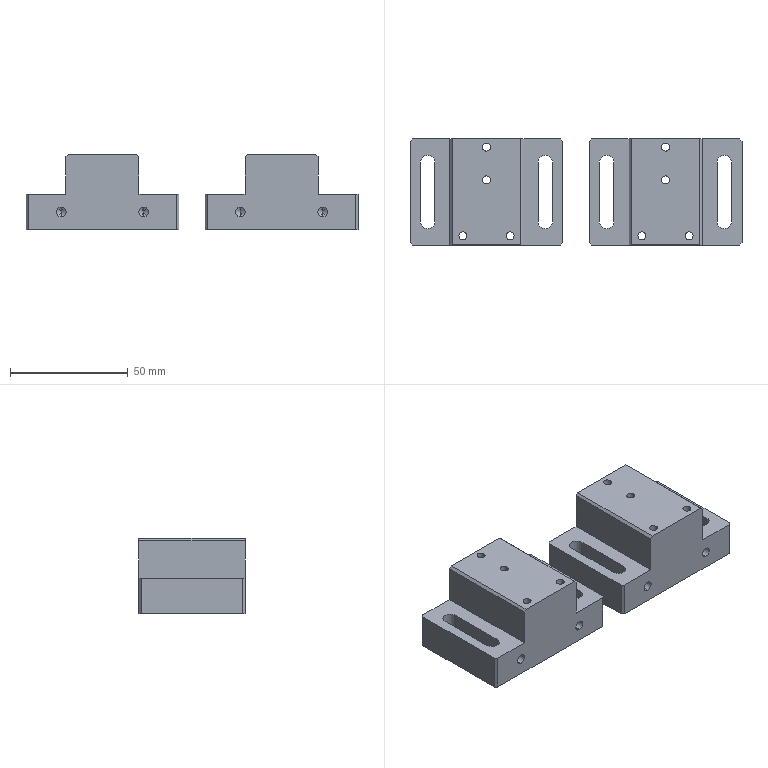NC program | NX | posted with a generic post | part box 140.92 x 45 x 32 mm
Lines 5945 to 6583 of 6583:
(FLOOR_WALL_1_COPY , TOOL : D10JING)
N11876 T14 M6
N11878 G54
N11880 G17 G0 G90 X-1.504 Y-6.448 S9500 M3
N11882 G43 Z30. H14
N11884 Z-15.5
N11886 G94 G1 Z-17. F1000.
N11888 X-0.497 Y-5.866
N11890 G3 X0.003 Y-5. R1.
N11892 G1 Y50. F1500.
N11894 X3.822
N11896 Y-5.
N11898 X7.641
N11900 Y50.
N11902 X11.46
N11904 Y-5.
N11906 G2 X10.96 Y-5.866 R1.
N11908 G1 X9.862 Y-6.5
N11910 Z-15.5
N11912 G0 X10.362
N11914 G1 Z-17. F1000.
N11916 X11.46 Y-5.866
N11918 G3 X11.96 Y-5. R1.
N11920 G1 Y50. F1500.
N11922 G3 X11.46 Y50.866 R1.
N11924 G1 X10.362 Y51.5
N11926 Z-15.5
N11928 G0 Z30.
N11930 X66.424 Y51.448
N11932 Z-15.5
N11934 G1 Z-17. F1000.
N11936 X65.417 Y50.866
N11938 G3 X64.917 Y50. R1.
N11940 G1 Y-5. F1500.
N11942 X61.098
N11944 Y50.
N11946 X57.279
N11948 Y-5.
N11950 X53.46
N11952 Y50.
N11954 G2 X53.96 Y50.866 R1.
N11956 G1 X55.058 Y51.5
N11958 Z-15.5
N11960 G0 X54.558
N11962 G1 Z-17. F1000.
N11964 X53.46 Y50.866
N11966 G3 X52.96 Y50. R1.
N11968 G1 Y-5. F1500.
N11970 G3 X53.46 Y-5.866 R1.
N11972 G1 X54.558 Y-6.5
N11974 Z-15.5
N11976 G0 Z30.
N11978 X74.496 Y-6.448
N11980 Z-15.5
N11982 G1 Z-17. F1000.
N11984 X75.503 Y-5.866
N11986 G3 X76.003 Y-5. R1.
N11988 G1 Y50. F1500.
N11990 X79.822
N11992 Y-5.
N11994 X83.641
N11996 Y50.
N11998 X87.46
N12000 Y-5.
N12002 G2 X86.96 Y-5.866 R1.
N12004 G1 X85.862 Y-6.5
N12006 Z-15.5
N12008 G0 X86.362
N12010 G1 Z-17. F1000.
N12012 X87.46 Y-5.866
N12014 G3 X87.96 Y-5. R1.
N12016 G1 Y50. F1500.
N12018 G3 X87.46 Y50.866 R1.
N12020 G1 X86.362 Y51.5
N12022 Z-15.5
N12024 G0 Z30.
N12026 X142.424 Y51.448
N12028 Z-15.5
N12030 G1 Z-17. F1000.
N12032 X141.417 Y50.866
N12034 G3 X140.917 Y50. R1.
N12036 G1 Y-5. F1500.
N12038 X137.098
N12040 Y50.
N12042 X133.279
N12044 Y-5.
N12046 X129.46
N12048 Y50.
N12050 G2 X129.96 Y50.866 R1.
N12052 G1 X131.058 Y51.5
N12054 Z-15.5
N12056 G0 X130.558
N12058 G1 Z-17. F1000.
N12060 X129.46 Y50.866
N12062 G3 X128.96 Y50. R1.
N12064 G1 Y-5. F1500.
N12066 G3 X129.46 Y-5.866 R1.
N12068 G1 X130.558 Y-6.5
N12070 Z-15.5
N12072 G0 Z30.
(ZLEVEL_PROFILE_1 , TOOL : D10JING)
N12074 X141.582 Y-6.809
N12076 Z-14.5
N12078 G1 Z-16. F1000.
N12080 X140.826 Y-5.5
N12082 G3 X139.96 Y-5. R1.
N12084 G1 X76.96 F1500.
N12086 G2 X73.424 Y-3.536 R5.
N12088 G1 X72.464 Y-2.576
N12090 G2 X71. Y0.96 R5.
N12092 G1 Y44.04
N12094 G2 X72.464 Y47.576 R5.
N12096 G1 X73.424 Y48.536
N12098 G2 X76.96 Y50. R5.
N12100 G1 X139.96
N12102 G2 X143.496 Y48.536 R5.
N12104 G1 X144.456 Y47.576
N12106 G2 X145.92 Y44.04 R5.
N12108 G1 Y0.96
N12110 G2 X144.456 Y-2.576 R5.
N12112 G1 X143.496 Y-3.536
N12114 G2 X139.96 Y-5. R5.
N12116 G3 X139.094 Y-5.5 R1.
N12118 G1 X138.228 Y-7.
N12120 Z-14.5
N12122 G0 Z30.
N12124 X65.582 Y-6.809
N12126 Z-14.5
N12128 G1 Z-16. F1000.
N12130 X64.826 Y-5.5
N12132 G3 X63.96 Y-5. R1.
N12134 G1 X0.96 F1500.
N12136 G2 X-2.576 Y-3.536 R5.
N12138 G1 X-3.536 Y-2.576
N12140 G2 X-5. Y0.96 R5.
N12142 G1 Y44.04
N12144 G2 X-3.536 Y47.576 R5.
N12146 G1 X-2.576 Y48.536
N12148 G2 X0.96 Y50. R5.
N12150 G1 X63.96
N12152 G2 X67.496 Y48.536 R5.
N12154 G1 X68.456 Y47.576
N12156 G2 X69.92 Y44.04 R5.
N12158 G1 Y0.96
N12160 G2 X68.456 Y-2.576 R5.
N12162 G1 X67.496 Y-3.536
N12164 G2 X63.96 Y-5. R5.
N12166 G1 X0.96 Z-20.048
N12168 X0.68 Y-4.992 Z-20.066
N12170 X0.4 Y-4.969 Z-20.084
N12172 X0.122 Y-4.929 Z-20.102
N12174 X-0.153 Y-4.875 Z-20.12
N12176 X-0.424 Y-4.805 Z-20.138
N12178 X-0.691 Y-4.719 Z-20.156
N12180 X-0.953 Y-4.619 Z-20.174
N12182 X-1.209 Y-4.505 Z-20.192
N12184 X-1.459 Y-4.376 Z-20.21
N12186 X-1.7 Y-4.234 Z-20.229
N12188 X-1.933 Y-4.078 Z-20.247
N12190 X-2.157 Y-3.909 Z-20.265
N12192 X-2.372 Y-3.728 Z-20.283
N12194 X-2.576 Y-3.536 Z-20.301
N12196 X-3.536 Y-2.576 Z-20.388
N12198 X-3.728 Y-2.372 Z-20.406
N12200 X-3.909 Y-2.157 Z-20.424
N12202 X-4.078 Y-1.933 Z-20.442
N12204 X-4.234 Y-1.7 Z-20.46
N12206 X-4.376 Y-1.459 Z-20.478
N12208 X-4.505 Y-1.209 Z-20.496
N12210 X-4.619 Y-0.953 Z-20.514
N12212 X-4.719 Y-0.691 Z-20.532
N12214 X-4.805 Y-0.424 Z-20.55
N12216 X-4.875 Y-0.153 Z-20.568
N12218 X-4.929 Y0.122 Z-20.586
N12220 X-4.969 Y0.4 Z-20.604
N12222 X-4.992 Y0.68 Z-20.622
N12224 X-5. Y0.96 Z-20.64
N12226 Y44.04 Z-23.408
N12228 X-4.992 Y44.32 Z-23.426
N12230 X-4.969 Y44.6 Z-23.444
N12232 X-4.929 Y44.878 Z-23.462
N12234 X-4.875 Y45.153 Z-23.48
N12236 X-4.805 Y45.424 Z-23.498
N12238 X-4.719 Y45.691 Z-23.516
N12240 X-4.619 Y45.953 Z-23.534
N12242 X-4.505 Y46.209 Z-23.552
N12244 X-4.376 Y46.459 Z-23.57
N12246 X-4.234 Y46.7 Z-23.588
N12248 X-4.078 Y46.933 Z-23.606
N12250 X-3.909 Y47.157 Z-23.625
N12252 X-3.728 Y47.372 Z-23.643
N12254 X-3.536 Y47.576 Z-23.661
N12256 X-2.576 Y48.536 Z-23.748
N12258 X-2.372 Y48.728 Z-23.766
N12260 X-2.157 Y48.909 Z-23.784
N12262 X-1.933 Y49.078 Z-23.802
N12264 X-1.7 Y49.234 Z-23.82
N12266 X-1.459 Y49.376 Z-23.838
N12268 X-1.209 Y49.505 Z-23.856
N12270 X-0.953 Y49.619 Z-23.874
N12272 X-0.691 Y49.719 Z-23.892
N12274 X-0.424 Y49.805 Z-23.91
N12276 X-0.153 Y49.875 Z-23.928
N12278 X0.122 Y49.929 Z-23.946
N12280 X0.4 Y49.969 Z-23.964
N12282 X0.68 Y49.992 Z-23.982
N12284 X0.96 Y50. Z-24.
N12286 X63.96 Z-28.048
N12288 X64.24 Y49.992 Z-28.066
N12290 X64.52 Y49.969 Z-28.084
N12292 X64.798 Y49.929 Z-28.102
N12294 X65.073 Y49.875 Z-28.12
N12296 X65.344 Y49.805 Z-28.138
N12298 X65.611 Y49.719 Z-28.156
N12300 X65.873 Y49.619 Z-28.174
N12302 X66.129 Y49.505 Z-28.192
N12304 X66.379 Y49.376 Z-28.21
N12306 X66.62 Y49.234 Z-28.229
N12308 X66.853 Y49.078 Z-28.247
N12310 X67.077 Y48.909 Z-28.265
N12312 X67.292 Y48.728 Z-28.283
N12314 X67.496 Y48.536 Z-28.301
N12316 X68.456 Y47.576 Z-28.388
N12318 X68.648 Y47.372 Z-28.406
N12320 X68.829 Y47.157 Z-28.424
N12322 X68.998 Y46.933 Z-28.442
N12324 X69.154 Y46.7 Z-28.46
N12326 X69.296 Y46.459 Z-28.478
N12328 X69.425 Y46.209 Z-28.496
N12330 X69.539 Y45.953 Z-28.514
N12332 X69.639 Y45.691 Z-28.532
N12334 X69.725 Y45.424 Z-28.55
N12336 X69.795 Y45.153 Z-28.568
N12338 X69.849 Y44.878 Z-28.586
N12340 X69.889 Y44.6 Z-28.604
N12342 X69.912 Y44.32 Z-28.622
N12344 X69.92 Y44.04 Z-28.64
N12346 Y0.96 Z-31.408
N12348 X69.912 Y0.68 Z-31.426
N12350 X69.889 Y0.4 Z-31.444
N12352 X69.849 Y0.122 Z-31.462
N12354 X69.795 Y-0.153 Z-31.48
N12356 X69.725 Y-0.424 Z-31.498
N12358 X69.639 Y-0.691 Z-31.516
N12360 X69.539 Y-0.953 Z-31.534
N12362 X69.425 Y-1.209 Z-31.552
N12364 X69.296 Y-1.459 Z-31.57
N12366 X69.154 Y-1.7 Z-31.588
N12368 X68.998 Y-1.933 Z-31.606
N12370 X68.829 Y-2.157 Z-31.625
N12372 X68.648 Y-2.372 Z-31.643
N12374 X68.456 Y-2.576 Z-31.661
N12376 X67.496 Y-3.536 Z-31.748
N12378 X67.292 Y-3.728 Z-31.766
N12380 X67.077 Y-3.909 Z-31.784
N12382 X66.853 Y-4.078 Z-31.802
N12384 X66.62 Y-4.234 Z-31.82
N12386 X66.379 Y-4.376 Z-31.838
N12388 X66.129 Y-4.505 Z-31.856
N12390 X65.873 Y-4.619 Z-31.874
N12392 X65.611 Y-4.719 Z-31.892
N12394 X65.344 Y-4.805 Z-31.91
N12396 X65.073 Y-4.875 Z-31.928
N12398 X64.798 Y-4.929 Z-31.946
N12400 X64.52 Y-4.969 Z-31.964
N12402 X64.24 Y-4.992 Z-31.982
N12404 X63.96 Y-5. Z-32.
N12406 X0.96
N12408 G2 X-2.576 Y-3.536 R5.
N12410 G1 X-3.536 Y-2.576
N12412 G2 X-5. Y0.96 R5.
N12414 G1 Y44.04
N12416 G2 X-3.536 Y47.576 R5.
N12418 G1 X-2.576 Y48.536
N12420 G2 X0.96 Y50. R5.
N12422 G1 X63.96
N12424 G2 X67.496 Y48.536 R5.
N12426 G1 X68.456 Y47.576
N12428 G2 X69.92 Y44.04 R5.
N12430 G1 Y0.96
N12432 G2 X68.456 Y-2.576 R5.
N12434 G1 X67.496 Y-3.536
N12436 G2 X63.96 Y-5. R5.
N12438 G3 X63.094 Y-5.5 R1.
N12440 G1 X62.228 Y-7.
N12442 Z-30.5
N12444 G0 Z30.
N12446 X141.582 Y-6.809
N12448 Z-30.5
N12450 G1 Z-32. F1000.
N12452 X140.826 Y-5.5
N12454 G3 X139.96 Y-5. R1.
N12456 G1 X76.96 F1500.
N12458 G2 X73.424 Y-3.536 R5.
N12460 G1 X72.464 Y-2.576
N12462 G2 X71. Y0.96 R5.
N12464 G1 Y44.04
N12466 G2 X72.464 Y47.576 R5.
N12468 G1 X73.424 Y48.536
N12470 G2 X76.96 Y50. R5.
N12472 G1 X139.96
N12474 G2 X143.496 Y48.536 R5.
N12476 G1 X144.456 Y47.576
N12478 G2 X145.92 Y44.04 R5.
N12480 G1 Y0.96
N12482 G2 X144.456 Y-2.576 R5.
N12484 G1 X143.496 Y-3.536
N12486 G2 X139.96 Y-5. R5.
N12488 G3 X139.094 Y-5.5 R1.
N12490 G1 X138.228 Y-7.
N12492 Z-30.5
N12494 G0 Z30.
N12496 M5
(DRILLING , TOOL : D6A45)
N12498 T01 M6
N12500 G54
N12502 G17 G0 G90 X108.46 Y41.5 S9500 M3
N12504 G43 Z30. H1
N12506 G94 G81 G98 Z-1.8 F250. R3.
N12508 Y27.6
N12510 X118.46 Y3.9
N12512 X98.46
N12514 X42.46
N12516 X22.46
N12518 X32.46 Y27.6
N12520 Y41.5
N12522 G80
N12524 G0 X32.46 Y41.5 Z30.
N12526 M5
(DRILLING_COPY_COPY , TOOL : 3.4ZT)
N12528 T16 M6
N12530 G54
N12532 G17 G0 G90 X108.46 Y41.5 S2000 M3
N12534 G43 Z30. H16
N12536 G94 G83 G98 Z-16.121 F150. Q2. R3.
N12538 Y27.6
N12540 X118.46 Y3.9
N12542 X98.46
N12544 X42.46
N12546 X22.46
N12548 X32.46 Y27.6
N12550 Y41.5
N12552 G80
N12554 G0 X32.46 Y41.5 Z30.
N12556 M5
(PLANAR_MILL_COPY , TOOL : D6A45)
N12558 T01 M6
N12560 G54
N12562 G17 G0 G90 X108.893 Y42.05 S9500 M3
N12564 G43 Z30. H1
N12566 Z0.5
N12568 G94 G1 Z-1. F1250.
N12570 G3 X108.46 Y42.3 R0.5
N12572 X107.66 Y41.5 R0.8
N12574 X108.46 Y42.3 R-0.8
N12576 X108.027 Y42.05 R0.5
N12578 G1 Z0.5
N12580 G0 Z30.
N12582 X109.01 Y27.167
N12584 Z0.5
N12586 G1 Z-1.
N12588 G3 X109.26 Y27.6 R0.5
N12590 X108.46 Y28.4 R0.8
N12592 X109.26 Y27.6 R-0.8
N12594 X109.01 Y28.033 R0.5
N12596 G1 Z0.5
N12598 G0 Z30.
N12600 X125.36 Y23.366
N12602 Z0.5
N12604 G1 Z-1.
N12606 G3 X124.86 Y22.5 R1.
N12608 G1 Y0.
N12610 G2 X123.96 Y-0.9 R0.9
N12612 G1 X92.96
N12614 G2 X92.06 Y0. R0.9
N12616 G1 Y45.
N12618 G2 X92.96 Y45.9 R0.9
N12620 G1 X123.96
N12622 G2 X124.86 Y45. R0.9
N12624 G1 Y22.5
N12626 G3 X125.36 Y21.634 R1.
N12628 G1 Z0.5
N12630 G0 Z30.
N12632 X118.027 Y3.35
N12634 Z0.5
N12636 G1 Z-1.
N12638 G3 X118.46 Y3.1 R0.5
N12640 X119.26 Y3.9 R0.8
N12642 X118.46 Y3.1 R-0.8
N12644 X118.893 Y3.35 R0.5
N12646 G1 Z0.5
N12648 G0 Z30.
N12650 X98.027
N12652 Z0.5
N12654 G1 Z-1.
N12656 G3 X98.46 Y3.1 R0.5
N12658 X99.26 Y3.9 R0.8
N12660 X98.46 Y3.1 R-0.8
N12662 X98.893 Y3.35 R0.5
N12664 G1 Z0.5
N12666 G0 Z30.
N12668 X42.027
N12670 Z0.5
N12672 G1 Z-1.
N12674 G3 X42.46 Y3.1 R0.5
N12676 X43.26 Y3.9 R0.8
N12678 X42.46 Y3.1 R-0.8
N12680 X42.893 Y3.35 R0.5
N12682 G1 Z0.5
N12684 G0 Z30.
N12686 X22.027
N12688 Z0.5
N12690 G1 Z-1.
N12692 G3 X22.46 Y3.1 R0.5
N12694 X23.26 Y3.9 R0.8
N12696 X22.46 Y3.1 R-0.8
N12698 X22.893 Y3.35 R0.5
N12700 G1 Z0.5
N12702 G0 Z30.
N12704 X15.56 Y21.634
N12706 Z0.5
N12708 G1 Z-1.
N12710 G3 X16.06 Y22.5 R1.
N12712 G1 Y45.
N12714 G2 X16.96 Y45.9 R0.9
N12716 G1 X47.96
N12718 G2 X48.86 Y45. R0.9
N12720 G1 Y0.
N12722 G2 X47.96 Y-0.9 R0.9
N12724 G1 X16.96
N12726 G2 X16.06 Y0. R0.9
N12728 G1 Y22.5
N12730 G3 X15.56 Y23.366 R1.
N12732 G1 Z0.5
N12734 G0 Z30.
N12736 X31.91 Y28.033
N12738 Z0.5
N12740 G1 Z-1.
N12742 G3 X31.66 Y27.6 R0.5
N12744 X32.46 Y26.8 R0.8
N12746 X31.66 Y27.6 R-0.8
N12748 X31.91 Y27.167 R0.5
N12750 G1 Z0.5
N12752 G0 Z30.
N12754 X32.893 Y42.05
N12756 Z0.5
N12758 G1 Z-1.
N12760 G3 X32.46 Y42.3 R0.5
N12762 X31.66 Y41.5 R0.8
N12764 X32.46 Y42.3 R-0.8
N12766 X32.027 Y42.05 R0.5
N12768 G1 Z0.5
N12770 G0 Z30.
(PLANAR_MILL_COPY_COPY , TOOL : D6A45)
N12772 X15.96 Y-0.866
N12774 Z0.
N12776 G1 Z-1.5
N12778 G3 X16.46 Y0. R1.
N12780 G1 Y45.
N12782 G3 X15.96 Y45.866 R1.
N12784 G1 Z0.
N12786 G0 Z30.
N12788 X48.96
N12790 Z0.
N12792 G1 Z-1.5
N12794 G3 X48.46 Y45. R1.
N12796 G1 Y0.
N12798 G3 X48.96 Y-0.866 R1.
N12800 G1 Z0.
N12802 G0 Z30.
N12804 X91.96
N12806 Z0.
N12808 G1 Z-1.5
N12810 G3 X92.46 Y0. R1.
N12812 G1 Y45.
N12814 G3 X91.96 Y45.866 R1.
N12816 G1 Z0.
N12818 G0 Z30.
N12820 X124.96
N12822 Z0.
N12824 G1 Z-1.5
N12826 G3 X124.46 Y45. R1.
N12828 G1 Y0.
N12830 G3 X124.96 Y-0.866 R1.
N12832 G1 Z0.
N12834 G0 Z30.
(PLANAR_MILL_COPY_COPY_1 , TOOL : D6A45)
N12836 X6.46 Y23.77
N12838 Z-16.5
N12840 G1 Z-18. F800.
N12842 X5.76 Y23.366
N12844 G3 X5.26 Y22.5 R1.
N12846 G1 Y10. F1250.
N12848 G3 X7.46 Y7.8 R2.2
N12850 X9.66 Y10. R2.2
N12852 G1 Y35.
N12854 G3 X7.46 Y37.2 R2.2
N12856 X5.26 Y35. R2.2
N12858 G1 Y22.5
N12860 G3 X5.76 Y21.634 R1.
N12862 G1 X6.46 Y21.23
N12864 Z-16.5
N12866 G0 Z30.
N12868 X56.46 Y23.77
N12870 Z-16.5
N12872 G1 Z-18. F800.
N12874 X55.76 Y23.366
N12876 G3 X55.26 Y22.5 R1.
N12878 G1 Y10. F1250.
N12880 G3 X57.46 Y7.8 R2.2
N12882 X59.66 Y10. R2.2
N12884 G1 Y35.
N12886 G3 X57.46 Y37.2 R2.2
N12888 X55.26 Y35. R2.2
N12890 G1 Y22.5
N12892 G3 X55.76 Y21.634 R1.
N12894 G1 X56.46 Y21.23
N12896 Z-16.5
N12898 G0 Z30.
N12900 X51.624 Y47.299
N12902 Z-16.5
N12904 G1 Z-18. F800.
N12906 X51.15 Y46.856
N12908 G3 X50.857 Y45.9 R1.
N12910 G1 X63.919 F1250.
N12912 G2 X64.626 Y45.607 R1.
N12914 G1 X65.527 Y44.706
N12916 G2 X65.82 Y43.999 R1.
N12918 G1 Y1.001
N12920 G2 X65.527 Y0.294 R1.
N12922 G1 X64.626 Y-0.607
N12924 G2 X63.919 Y-0.9 R1.
N12926 G1 X50.857
N12928 G3 X51.15 Y-1.856 R1.
N12930 G1 X51.624 Y-2.299
N12932 Z-16.5
N12934 G0 Z30.
N12936 X13.296
N12938 Z-16.5
N12940 G1 Z-18. F800.
N12942 X13.77 Y-1.856
N12944 G3 X14.063 Y-0.9 R1.
N12946 G1 X1.001 F1250.
N12948 G2 X0.294 Y-0.607 R1.
N12950 G1 X-0.607 Y0.294
N12952 G2 X-0.9 Y1.001 R1.
N12954 G1 Y43.999
N12956 G2 X-0.607 Y44.706 R1.
N12958 G1 X0.294 Y45.607
N12960 G2 X1.001 Y45.9 R1.
N12962 G1 X14.063
N12964 G3 X13.77 Y46.856 R1.
N12966 G1 X13.296 Y47.299
N12968 Z-16.5
N12970 G0 Z30.
N12972 X89.296 Y-2.299
N12974 Z-16.5
N12976 G1 Z-18. F800.
N12978 X89.77 Y-1.856
N12980 G3 X90.063 Y-0.9 R1.
N12982 G1 X77.001 F1250.
N12984 G2 X76.294 Y-0.607 R1.
N12986 G1 X75.393 Y0.294
N12988 G2 X75.1 Y1.001 R1.
N12990 G1 Y43.999
N12992 G2 X75.393 Y44.706 R1.
N12994 G1 X76.294 Y45.607
N12996 G2 X77.001 Y45.9 R1.
N12998 G1 X90.063
N13000 G3 X89.77 Y46.856 R1.
N13002 G1 X89.296 Y47.299
N13004 Z-16.5
N13006 G0 Z30.
N13008 X127.624
N13010 Z-16.5
N13012 G1 Z-18. F800.
N13014 X127.15 Y46.856
N13016 G3 X126.857 Y45.9 R1.
N13018 G1 X139.919 F1250.
N13020 G2 X140.626 Y45.607 R1.
N13022 G1 X141.527 Y44.706
N13024 G2 X141.82 Y43.999 R1.
N13026 G1 Y1.001
N13028 G2 X141.527 Y0.294 R1.
N13030 G1 X140.626 Y-0.607
N13032 G2 X139.919 Y-0.9 R1.
N13034 G1 X126.857
N13036 G3 X127.15 Y-1.856 R1.
N13038 G1 X127.624 Y-2.299
N13040 Z-16.5
N13042 G0 Z30.
N13044 X82.46 Y23.77
N13046 Z-16.5
N13048 G1 Z-18. F800.
N13050 X81.76 Y23.366
N13052 G3 X81.26 Y22.5 R1.
N13054 G1 Y10. F1250.
N13056 G3 X83.46 Y7.8 R2.2
N13058 X85.66 Y10. R2.2
N13060 G1 Y35.
N13062 G3 X83.46 Y37.2 R2.2
N13064 X81.26 Y35. R2.2
N13066 G1 Y22.5
N13068 G3 X81.76 Y21.634 R1.
N13070 G1 X82.46 Y21.23
N13072 Z-16.5
N13074 G0 Z30.
N13076 X134.46
N13078 Z-16.5
N13080 G1 Z-18. F800.
N13082 X135.16 Y21.634
N13084 G3 X135.66 Y22.5 R1.
N13086 G1 Y35. F1250.
N13088 G3 X133.46 Y37.2 R2.2
N13090 X131.26 Y35. R2.2
N13092 G1 Y10.
N13094 G3 X133.46 Y7.8 R2.2
N13096 X135.66 Y10. R2.2
N13098 G1 Y22.5
N13100 G3 X135.16 Y23.366 R1.
N13102 G1 X134.46 Y23.77
N13104 Z-16.5
N13106 G0 Z30.
N13108 M5
N13110 M2